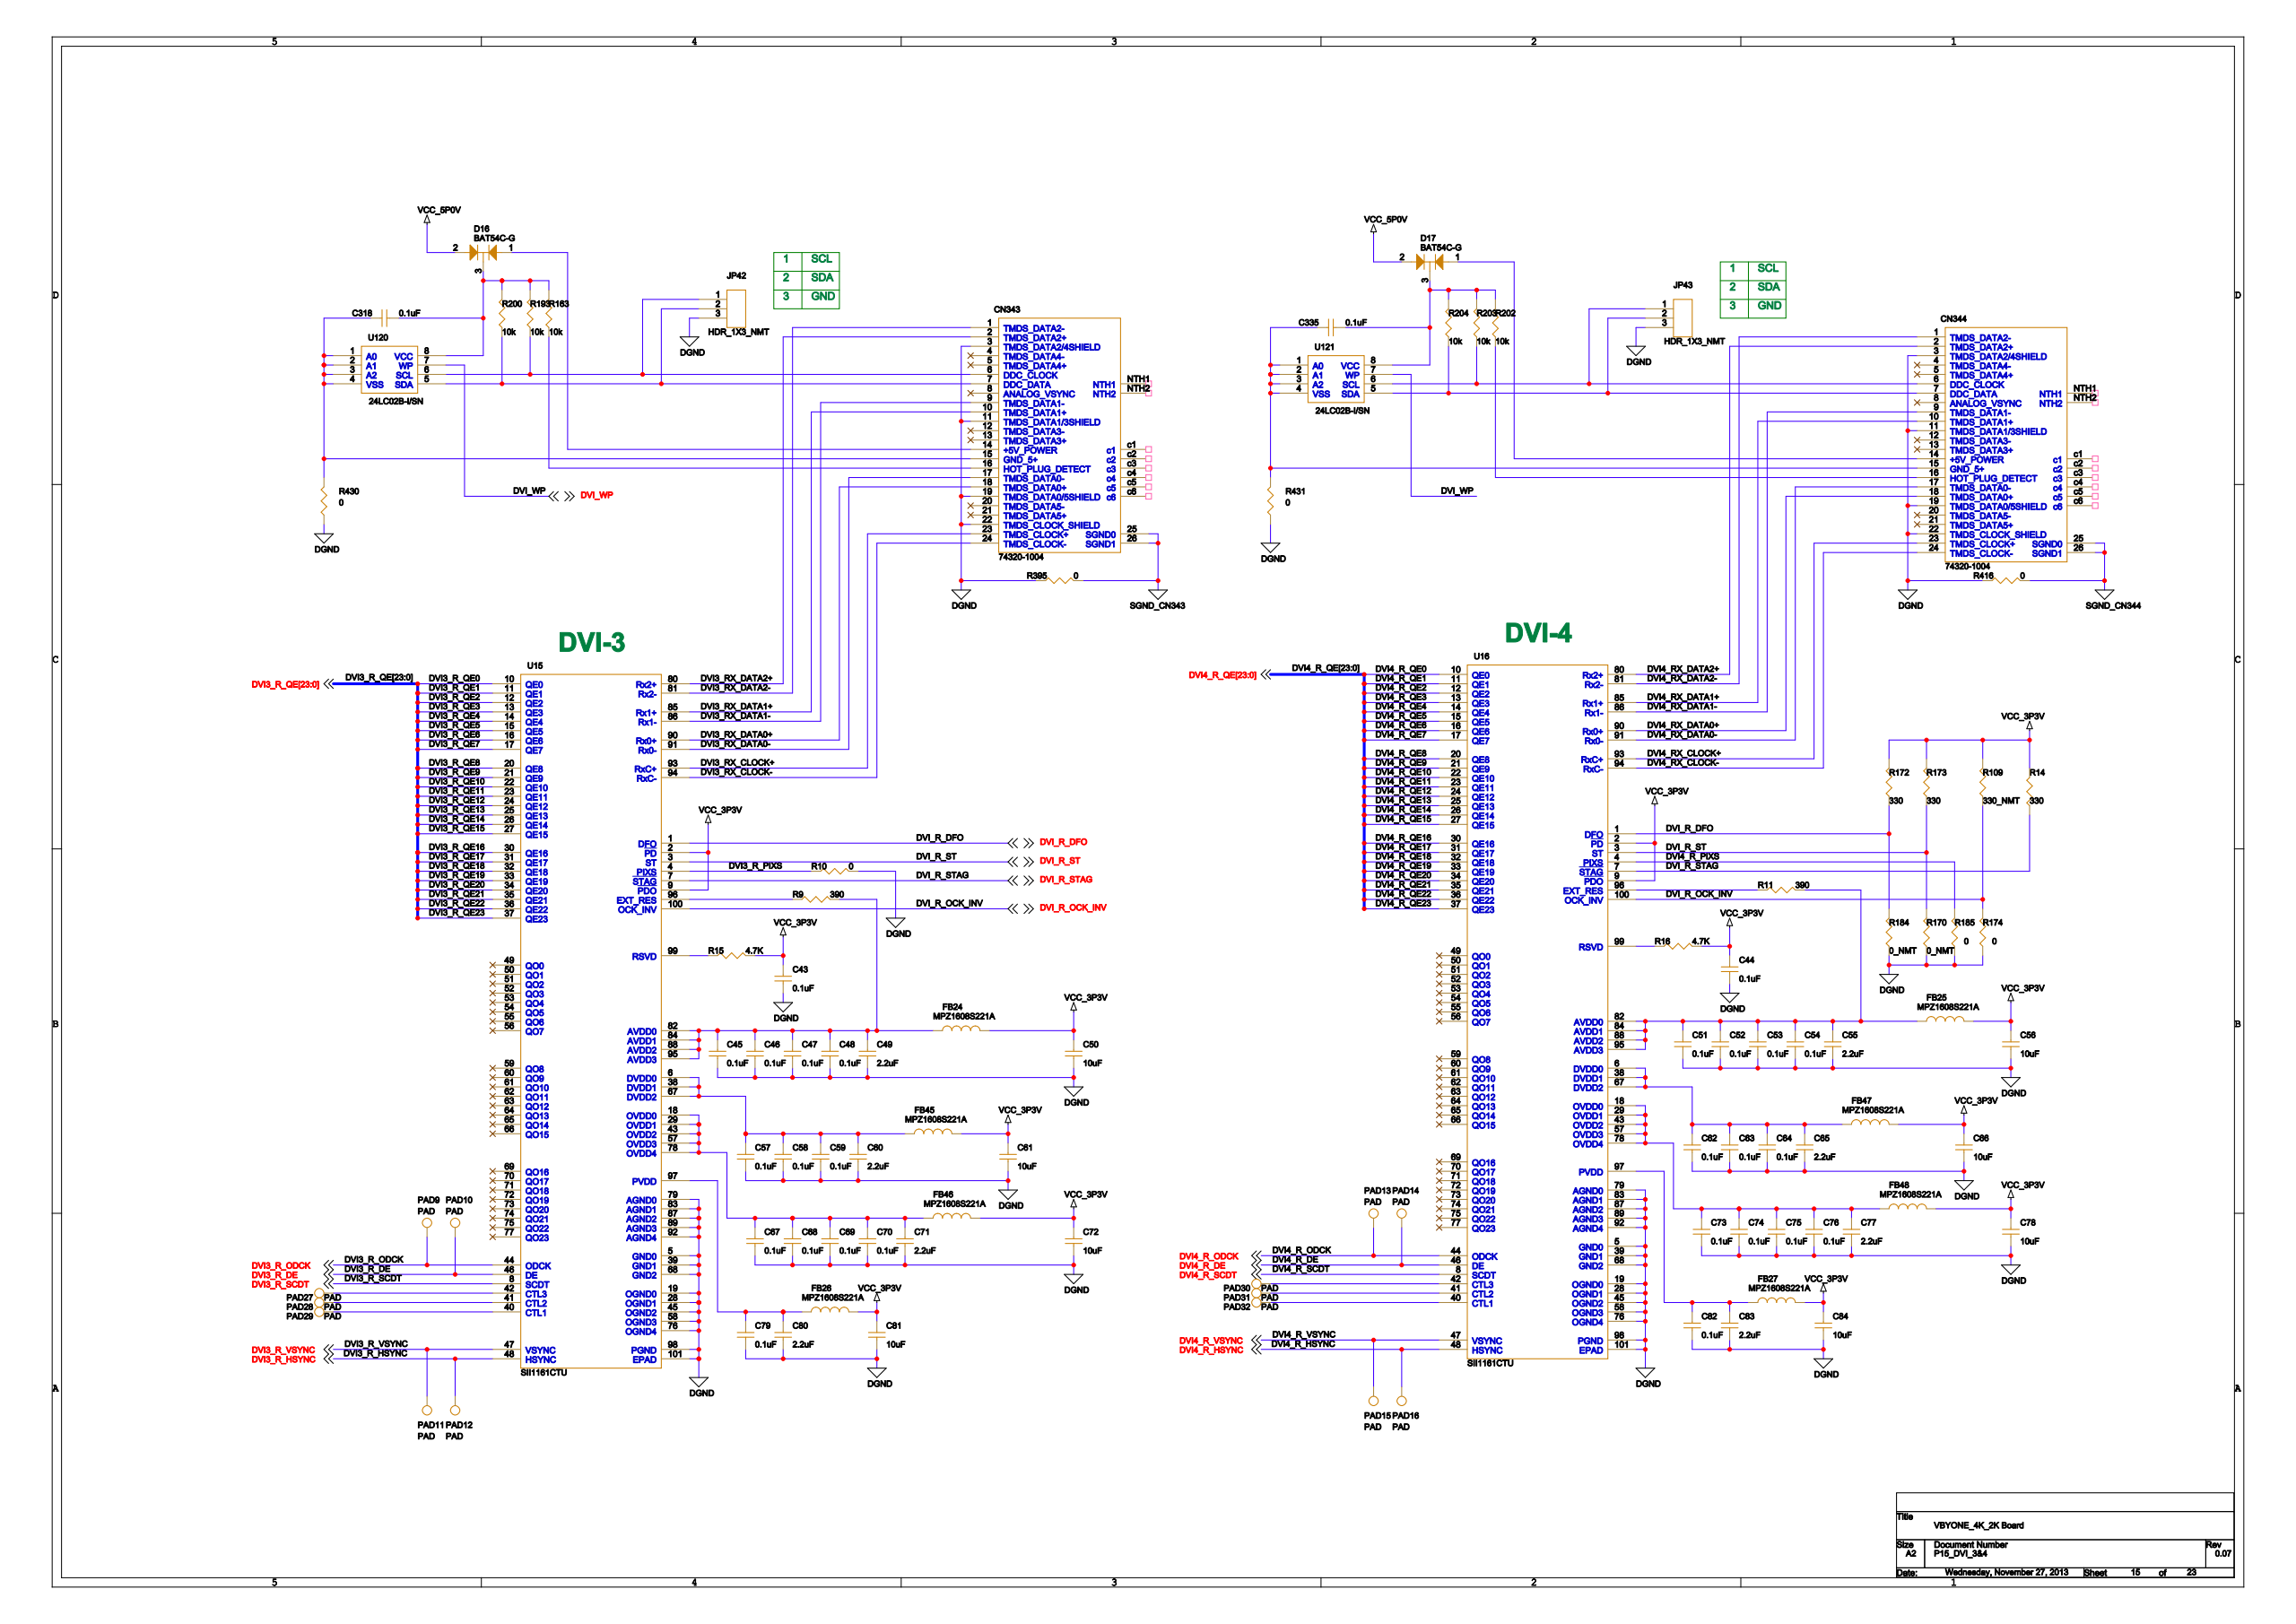Circuit board | Cadence Allegro | 1712 parts | 1495 nets | one sheet of the schematic
Parts on this sheet (reference | value | footprint):
C43 | 0.1uF | CRC1005RZAS
C44 | 0.1uF | CRC1005RZAS
C45 | 0.1uF | CRC1005RZAS
C46 | 0.1uF | CRC1005RZAS
C47 | 0.1uF | CRC1005RZAS
C48 | 0.1uF | CRC1005RZAS
C49 | 2.2uF | CRC1608RZAS
C50 | 10uF | CRC2012RZAS
C51 | 0.1uF | CRC1005RZAS
C52 | 0.1uF | CRC1005RZAS
C53 | 0.1uF | CRC1005RZAS
C54 | 0.1uF | CRC1005RZAS
C55 | 2.2uF | CRC1608RZAS
C56 | 10uF | CRC2012RZAS
C57 | 0.1uF | CRC1005RZAS
C58 | 0.1uF | CRC1005RZAS
C59 | 0.1uF | CRC1005RZAS
C60 | 2.2uF | CRC1608RZAS
C61 | 10uF | CRC2012RZAS
C62 | 0.1uF | CRC1005RZAS
C63 | 0.1uF | CRC1005RZAS
C64 | 0.1uF | CRC1005RZAS
C65 | 2.2uF | CRC1608RZAS
C66 | 10uF | CRC2012RZAS
C67 | 0.1uF | CRC1005RZAS
C68 | 0.1uF | CRC1005RZAS
C69 | 0.1uF | CRC1005RZAS
C70 | 0.1uF | CRC1005RZAS
C71 | 2.2uF | CRC1608RZAS
C72 | 10uF | CRC2012RZAS
C73 | 0.1uF | CRC1005RZAS
C74 | 0.1uF | CRC1005RZAS
C75 | 0.1uF | CRC1005RZAS
C76 | 0.1uF | CRC1005RZAS
C77 | 2.2uF | CRC1608RZAS
C78 | 10uF | CRC2012RZAS
C79 | 0.1uF | CRC1005RZAS
C80 | 2.2uF | CRC1608RZAS
C81 | 10uF | CRC2012RZAS
C82 | 0.1uF | CRC1005RZAS
C83 | 2.2uF | CRC1608RZAS
C84 | 10uF | CRC2012RZAS
C318 | 0.1uF | CRC1005RZAS
C335 | 0.1uF | CRC1005RZAS
CN343 | 74320-1004 | CAD030LZAS
CN344 | 74320-1004 | CAD030LZAS
D16 | BAT54C-G | DIC003RZCS
D17 | BAT54C-G | DIC003RZCS
FB24 | MPZ1608S221A | LSC1608RZAS
FB25 | MPZ1608S221A | LSC1608RZAS
FB26 | MPZ1608S221A | LSC1608RZAS
FB27 | MPZ1608S221A | LSC1608RZAS
FB45 | MPZ1608S221A | LSC1608RZAS
FB46 | MPZ1608S221A | LSC1608RZAS
FB47 | MPZ1608S221A | LSC1608RZAS
FB48 | MPZ1608S221A | LSC1608RZAS
JP42 | HDR_1X3_NMT | CND003LLBS
JP43 | HDR_1X3_NMT | CND003LLBS
PAD9 | PAD | TPC050
PAD10 | PAD | TPC050
PAD11 | PAD | TPC050
PAD12 | PAD | TPC050
PAD13 | PAD | TPC050
PAD14 | PAD | TPC050
PAD15 | PAD | TPC050
PAD16 | PAD | TPC050
PAD27 | PAD | TPC050
PAD28 | PAD | TPC050
PAD29 | PAD | TPC050
PAD30 | PAD | TPC050
PAD31 | PAD | TPC050
PAD32 | PAD | TPC050
R9 | 390 | CRC1608RZAS
R10 | 0 | CRC1608RZAS
R11 | 390 | CRC1608RZAS
R14 | 330 | CRC1608RZAS
R16 | 4.7K | CRC1005RZAS
R109 | 330_NMT | CRC1608RZAS
R163 | 10K | CRC1005RZAS
R170 | 0_NMT | CRC1608RZAS
R172 | 330 | CRC1608RZAS
R173 | 330 | CRC1608RZAS
R174 | 0 | CRC1608RZAS
R184 | 0_NMT | CRC1608RZAS
R185 | 0 | CRC1608RZAS
R193 | 10K | CRC1005RZAS
R200 | 10K | CRC1005RZAS
R202 | 10K | CRC1005RZAS
R203 | 10K | CRC1005RZAS
R204 | 10K | CRC1005RZAS
R395 | 0 | CRC1608RZAS
R416 | 0 | CRC1608RZAS
R430 | 0 | CRC1608RZAS
R431 | 0 | CRC1608RZAS
U15 | SII1161CTU | QFP100RCBS
U16 | SII1161CTU | QFP100RCBS
U120 | 24LC02B-I/SN | SOC008RHDS
U121 | 24LC02B-I/SN | SOC008RHDS
Nets of these parts (net: part-pin ...):
VCC_3P3V: C43-1 C44-1 C50-1 C56-1 C61-1 C66-1 C72-1 C78-1 C81-1 C84-1 FB24-2 FB25-2 FB26-2 FB27-2 FB45-2 FB46-2 FB47-2 FB48-2 R14-2 R16-2 R109-2 R172-2 R173-2 U15-2 U15-9 U16-2 U16-9
DGND: C43-2 C44-2 C45-2 C46-2 C47-2 C48-2 C49-2 C50-2 C51-2 C52-2 C53-2 C54-2 C55-2 C56-2 C57-2 C58-2 C59-2 C60-2 C61-2 C62-2 C63-2 C64-2 C65-2 C66-2 C67-2 C68-2 C69-2 C70-2 C71-2 C72-2 C73-2 C74-2 C75-2 C76-2 C77-2 C78-2 C79-2 C80-2 C81-2 C82-2 C83-2 C84-2 CN343-3 CN343-11 CN343-19 CN343-22 CN344-3 CN344-11 CN344-19 CN344-22 JP42-3 JP43-3 R10-2 R170-1 R174-1 R184-1 R185-1 R395-1 R416-1 R430-1 R431-1 U15-5 U15-19 U15-28 U15-39 U15-45 U15-58 U15-68 U15-76 U15-79 U15-83 U15-87 U15-89 U15-92 U15-98 U15-101 U16-5 U16-19 U16-28 U16-39 U16-45 U16-58 U16-68 U16-76 U16-79 U16-83 U16-87 U16-89 U16-92 U16-98 U16-101
N18926970: C318-1 CN343-15 R430-2 U120-1 U120-2 U120-3 U120-4
N18926978: C318-2 D16-3 R163-2 R193-2 R200-2 U120-8
N18927955: C335-1 CN344-15 R431-2 U121-1 U121-2 U121-3 U121-4
N18927963: C335-2 D17-3 R202-2 R203-2 R204-2 U121-8
N15921230: C45-1 C46-1 C47-1 C48-1 C49-1 FB24-1 R9-2 U15-82 U15-84 U15-88 U15-95
N15919632: C51-1 C52-1 C53-1 C54-1 C55-1 FB25-1 R11-2 U16-82 U16-84 U16-88 U16-95
N15918608: C57-1 C58-1 C59-1 C60-1 FB45-1 U15-6 U15-38 U15-67
N15918088: C62-1 C63-1 C64-1 C65-1 FB47-1 U16-6 U16-38 U16-67
N15918006: C67-1 C68-1 C69-1 C70-1 C71-1 FB46-1 U15-18 U15-29 U15-43 U15-57 U15-78
N15918056: C73-1 C74-1 C75-1 C76-1 C77-1 FB48-1 U16-18 U16-29 U16-43 U16-57 U16-78
N15922124: C79-1 C80-1 FB26-1 U15-97
N15920652: C82-1 C83-1 FB27-1 U16-97
VCC_5P0V: D16-2 D17-2
SGND_CN343: CN343-25 CN343-26 R395-2
DVI3_RX_DATA0-: CN343-17 U15-91
DVI3_RX_DATA1-: CN343-9 U15-86
DVI3_RX_DATA2-: CN343-1 U15-81
DVI3_RX_DATA0+: CN343-18 U15-90
DVI3_RX_DATA1+: CN343-10 U15-85
DVI3_RX_DATA2+: CN343-2 U15-80
N18926974: CN343-14 D16-1
N18926991: CN343-6 JP42-1 R193-1 U120-6
DVI3_RX_CLOCK+: CN343-23 U15-93
N18926997: CN343-7 JP42-2 R200-1 U120-5
DVI3_RX_CLOCK-: CN343-24 U15-94
N18927190: CN343-16 R163-1
SGND_CN344: CN344-25 CN344-26 R416-2
DVI4_RX_DATA0-: CN344-17 U16-91
DVI4_RX_DATA1-: CN344-9 U16-86
DVI4_RX_DATA2-: CN344-1 U16-81
DVI4_RX_DATA0+: CN344-18 U16-90
DVI4_RX_DATA1+: CN344-10 U16-85
DVI4_RX_DATA2+: CN344-2 U16-80
N18927959: CN344-14 D17-1
N18927976: CN344-6 JP43-1 R203-1 U121-6
DVI4_RX_CLOCK+: CN344-23 U16-93
N18927982: CN344-7 JP43-2 R204-1 U121-5
DVI4_RX_CLOCK-: CN344-24 U16-94
N18928175: CN344-16 R202-1
DVI_WP: U120-7 U121-7
DVI3_R_DE: PAD10-1 U15-46
DVI3_R_VSYNC: PAD11-1 U15-47
DVI3_R_HSYNC: PAD12-1 U15-48
DVI4_R_ODCK: PAD13-1 U16-44
DVI4_R_DE: PAD14-1 U16-46
DVI4_R_VSYNC: PAD15-1 U16-47
DVI4_R_HSYNC: PAD16-1 U16-48
N19424426: PAD27-1 U15-42
N19424444: PAD28-1 U15-41
N19424442: PAD29-1 U15-40
N19424489: PAD30-1 U16-42
N19424507: PAD31-1 U16-41
N19424505: PAD32-1 U16-40
DVI3_R_ODCK: PAD9-1 U15-44
DVI3_R_PIXS: R10-1 U15-4
DVI_R_OCK_INV: R109-1 R174-2 U15-100 U16-100
DVI4_R_PIXS: R185-2 U16-4
N15919696: R16-1 U16-99
DVI_R_ST: R170-2 R173-1 U15-3 U16-3
DVI_R_DFO: R172-1 R184-2 U15-1 U16-1
N19369828: R11-1 U16-96
N19369419: R9-1 U15-96
DVI_R_STAG: R14-1 U15-7 U16-7
DVI3_R_SCDT: U15-8
DVI3_R_QE0: U15-10
DVI3_R_QE2: U15-12
DVI3_R_QE1: U15-11
DVI3_R_QE3: U15-13
DVI3_R_QE4: U15-14
DVI3_R_QE6: U15-16
DVI3_R_QE5: U15-15
DVI3_R_QE7: U15-17
DVI3_R_QE8: U15-20
DVI3_R_QE9: U15-21
DVI3_R_QE10: U15-22
DVI3_R_QE12: U15-24
DVI3_R_QE11: U15-23
DVI3_R_QE13: U15-25
DVI3_R_QE14: U15-26
DVI3_R_QE15: U15-27
DVI3_R_QE16: U15-30
DVI3_R_QE17: U15-31
DVI3_R_QE19: U15-33
DVI3_R_QE18: U15-32
DVI3_R_QE20: U15-34
DVI3_R_QE21: U15-35
DVI3_R_QE23: U15-37
DVI3_R_QE22: U15-36
DVI4_R_SCDT: U16-8
DVI4_R_QE0: U16-10
DVI4_R_QE2: U16-12
DVI4_R_QE1: U16-11
DVI4_R_QE3: U16-13
DVI4_R_QE4: U16-14
DVI4_R_QE6: U16-16
DVI4_R_QE5: U16-15
DVI4_R_QE7: U16-17
DVI4_R_QE8: U16-20
DVI4_R_QE9: U16-21
DVI4_R_QE10: U16-22
DVI4_R_QE12: U16-24
DVI4_R_QE11: U16-23
DVI4_R_QE13: U16-25
DVI4_R_QE14: U16-26
DVI4_R_QE15: U16-27
DVI4_R_QE16: U16-30
DVI4_R_QE17: U16-31
DVI4_R_QE19: U16-33
DVI4_R_QE18: U16-32
DVI4_R_QE20: U16-34
DVI4_R_QE21: U16-35
DVI4_R_QE23: U16-37
DVI4_R_QE22: U16-36